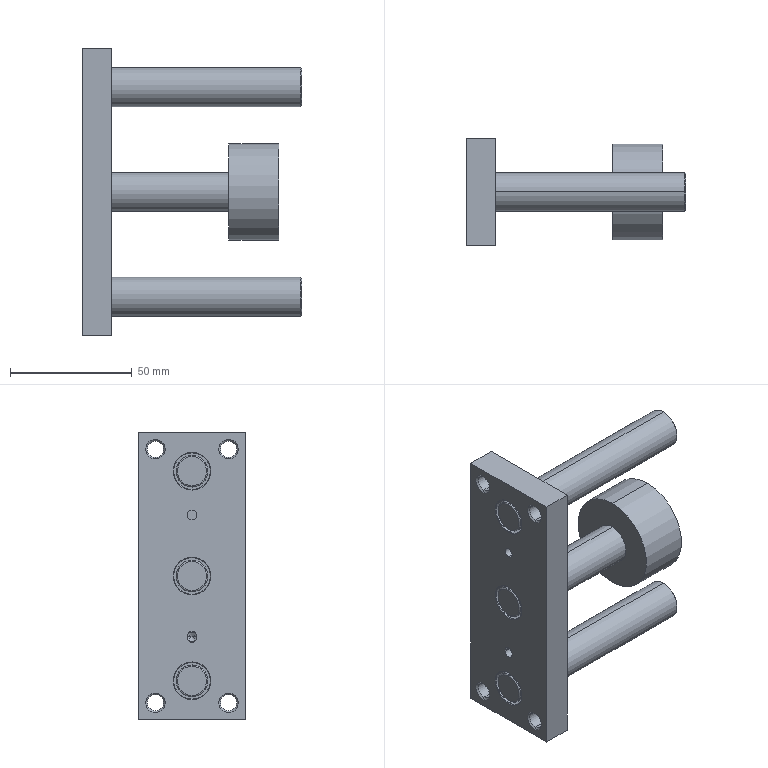Part | SolidWorks | features BaseBody 1 | 1 solid | 90 faces | box 90 x 44 x 118 mm | volume 125856 mm3 | cylinder 35 | cone 28 | plane 21 | torus 6 | commonest cylinder face diameters 6.647 x8 4 x7 13 x6 15 x6 16 x6 39.6 x2